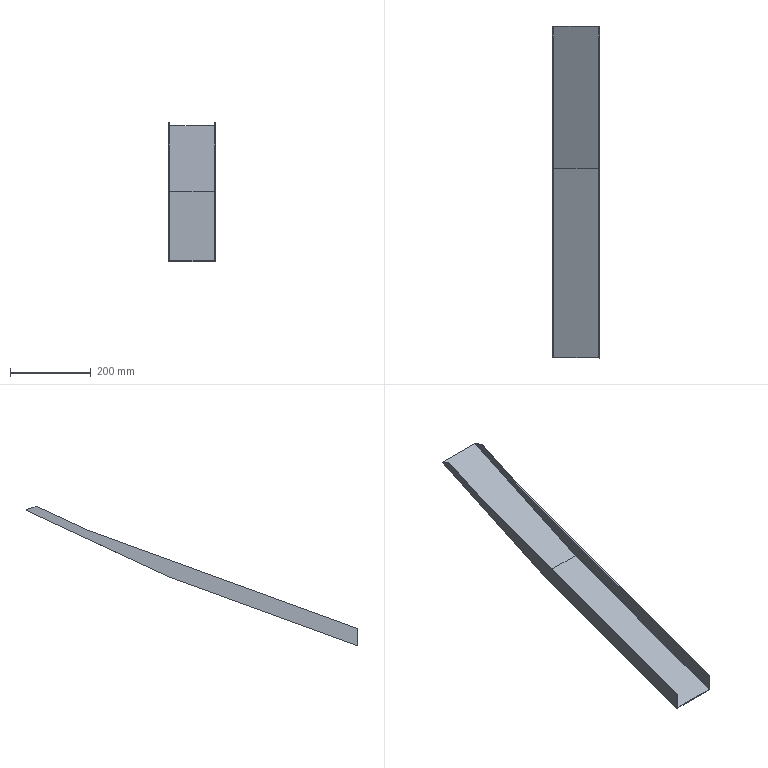Part | NX | features solid 2 | 1 solid | 16 faces | box 115.013 x 820.651 x 345.175 mm | volume 314941 mm3 | plane 16
STEP:
#1=CARTESIAN_POINT('',(53.,-0.1941,-173.187));
#2=VERTEX_POINT('',#1);
#3=CARTESIAN_POINT('',(-60.,-0.1961,-173.178));
#4=VERTEX_POINT('',#3);
#5=CARTESIAN_POINT('',(55.,-0.194,-173.187));
#6=DIRECTION('',(-1.,-0.00001764,0.00007989));
#7=VECTOR('',#6,1000.);
#8=LINE('',#5,#7);
#9=EDGE_CURVE('',#2,#4,#8,.T.);
#10=ORIENTED_EDGE('',*,*,#9,.F.);
#11=CARTESIAN_POINT('',(55.,-0.194,-173.187));
#12=VERTEX_POINT('',#11);
#13=CARTESIAN_POINT('',(55.,-0.194,-173.187));
#14=DIRECTION('',(-1.,-0.00001764,0.00007989));
#15=VECTOR('',#14,1000.);
#16=LINE('',#13,#15);
#17=EDGE_CURVE('',#12,#2,#16,.T.);
#18=ORIENTED_EDGE('',*,*,#17,.F.);
#19=CARTESIAN_POINT('',(55.,0.6512,-175.));
#20=VERTEX_POINT('',#19);
#21=CARTESIAN_POINT('',(54.999,6.339,-187.197));
#22=DIRECTION('',(-0.00008156,0.4226,-0.9063));
#23=VECTOR('',#22,1000.);
#24=LINE('',#21,#23);
#25=EDGE_CURVE('',#12,#20,#24,.T.);
#26=ORIENTED_EDGE('',*,*,#25,.T.);
#27=CARTESIAN_POINT('',(-60.,0.6492,-174.991));
#28=VERTEX_POINT('',#27);
#29=CARTESIAN_POINT('',(55.,0.6512,-175.));
#30=DIRECTION('',(-1.,-0.00001764,0.00007989));
#31=VECTOR('',#30,1000.);
#32=LINE('',#29,#31);
#33=EDGE_CURVE('',#20,#28,#32,.T.);
#34=ORIENTED_EDGE('',*,*,#33,.T.);
#35=CARTESIAN_POINT('',(-60.001,6.337,-187.187));
#36=DIRECTION('',(-0.00008156,0.4226,-0.9063));
#37=VECTOR('',#36,1000.);
#38=LINE('',#35,#37);
#39=EDGE_CURVE('',#4,#28,#38,.T.);
#40=ORIENTED_EDGE('',*,*,#39,.F.);
#41=EDGE_LOOP('',(#10,#18,#26,#34,#40));
#42=FACE_BOUND('',#41,.T.);
#43=CARTESIAN_POINT('',(55.,0.6512,-175.));
#44=DIRECTION('',(-0.00001778,-0.9063,-0.4226));
#45=DIRECTION('',(-1.,-0.00001836,0.00008143));
#46=AXIS2_PLACEMENT_3D('',#43,#44,#45);
#47=PLANE('',#46);
#48=ADVANCED_FACE('',(#42),#47,.F.);
#49=CARTESIAN_POINT('',(-60.007,-350.766,-338.858));
#50=VERTEX_POINT('',#49);
#51=CARTESIAN_POINT('',(-60.004,-190.561,-264.153));
#52=DIRECTION('',(-0.00001778,-0.9063,-0.4226));
#53=VECTOR('',#52,1000.);
#54=LINE('',#51,#53);
#55=EDGE_CURVE('',#28,#50,#54,.T.);
#56=ORIENTED_EDGE('',*,*,#55,.T.);
#57=CARTESIAN_POINT('',(-60.012,-820.,-509.646));
#58=VERTEX_POINT('',#57);
#59=CARTESIAN_POINT('',(-60.005,-184.189,-278.229));
#60=DIRECTION('',(-0.0000106,-0.9397,-0.342));
#61=VECTOR('',#60,1000.);
#62=LINE('',#59,#61);
#63=EDGE_CURVE('',#58,#50,#62,.F.);
#64=ORIENTED_EDGE('',*,*,#63,.F.);
#65=CARTESIAN_POINT('',(-60.009,-820.,-467.078));
#66=VERTEX_POINT('',#65);
#67=CARTESIAN_POINT('',(-60.028,-820.,-699.908));
#68=DIRECTION('',(-0.00008143,0.,-1.));
#69=VECTOR('',#68,1000.);
#70=LINE('',#67,#69);
#71=EDGE_CURVE('',#58,#66,#70,.F.);
#72=ORIENTED_EDGE('',*,*,#71,.T.);
#73=CARTESIAN_POINT('',(-60.001,-150.453,-223.383));
#74=VERTEX_POINT('',#73);
#75=CARTESIAN_POINT('',(-60.002,-197.87,-240.642));
#76=DIRECTION('',(0.0000106,0.9397,0.342));
#77=VECTOR('',#76,1000.);
#78=LINE('',#75,#77);
#79=EDGE_CURVE('',#66,#74,#78,.T.);
#80=ORIENTED_EDGE('',*,*,#79,.T.);
#81=CARTESIAN_POINT('',(-59.999,-24.136,-164.481));
#82=VERTEX_POINT('',#81);
#83=CARTESIAN_POINT('',(-59.998,-7.823,-156.874));
#84=DIRECTION('',(-0.00001778,-0.9063,-0.4226));
#85=VECTOR('',#84,1000.);
#86=LINE('',#83,#85);
#87=EDGE_CURVE('',#82,#74,#86,.T.);
#88=ORIENTED_EDGE('',*,*,#87,.F.);
#89=CARTESIAN_POINT('',(-60.,-0.2158,-173.187));
#90=VERTEX_POINT('',#89);
#91=CARTESIAN_POINT('',(-59.97,-615.968,50.928));
#92=DIRECTION('',(-0.0000451,0.9397,-0.342));
#93=VECTOR('',#92,1000.);
#94=LINE('',#91,#93);
#95=EDGE_CURVE('',#82,#90,#94,.T.);
#96=ORIENTED_EDGE('',*,*,#95,.T.);
#97=CARTESIAN_POINT('',(-60.004,-191.406,-262.341));
#98=DIRECTION('',(-0.00001778,-0.9063,-0.4226));
#99=VECTOR('',#98,1000.);
#100=LINE('',#97,#99);
#101=EDGE_CURVE('',#4,#90,#100,.T.);
#102=ORIENTED_EDGE('',*,*,#101,.F.);
#103=ORIENTED_EDGE('',*,*,#39,.T.);
#104=EDGE_LOOP('',(#56,#64,#72,#80,#88,#96,#102,#103));
#105=FACE_BOUND('',#104,.T.);
#106=CARTESIAN_POINT('',(-60.005,-184.873,-276.35));
#107=DIRECTION('',(1.,0.00001836,-0.00008143));
#108=DIRECTION('',(-0.00008143,0.,-1.));
#109=AXIS2_PLACEMENT_3D('',#106,#107,#108);
#110=PLANE('',#109);
#111=ADVANCED_FACE('',(#105),#110,.F.);
#112=CARTESIAN_POINT('',(-58.007,-350.766,-338.859));
#113=VERTEX_POINT('',#112);
#114=CARTESIAN_POINT('',(-60.007,-350.766,-338.858));
#115=CARTESIAN_POINT('',(-59.34,-350.766,-338.858));
#116=CARTESIAN_POINT('',(-58.674,-350.766,-338.859));
#117=CARTESIAN_POINT('',(-58.007,-350.766,-338.859));
#118=B_SPLINE_CURVE_WITH_KNOTS('',3,(#114,#115,#116,#117),.UNSPECIFIED.,.F.,.F.,(4,4),(0.,1.),.UNSPECIFIED.);
#119=EDGE_CURVE('',#50,#113,#118,.T.);
#120=ORIENTED_EDGE('',*,*,#119,.T.);
#121=CARTESIAN_POINT('',(52.993,-350.766,-338.868));
#122=VERTEX_POINT('',#121);
#123=CARTESIAN_POINT('',(64.99,-350.766,-338.869));
#124=DIRECTION('',(1.,0.,-0.00008812));
#125=VECTOR('',#124,1000.);
#126=LINE('',#123,#125);
#127=EDGE_CURVE('',#113,#122,#126,.T.);
#128=ORIENTED_EDGE('',*,*,#127,.T.);
#129=CARTESIAN_POINT('',(54.993,-350.766,-338.869));
#130=VERTEX_POINT('',#129);
#131=CARTESIAN_POINT('',(52.993,-350.766,-338.868));
#132=CARTESIAN_POINT('',(53.66,-350.766,-338.868));
#133=CARTESIAN_POINT('',(54.326,-350.766,-338.869));
#134=CARTESIAN_POINT('',(54.993,-350.766,-338.869));
#135=B_SPLINE_CURVE_WITH_KNOTS('',3,(#131,#132,#133,#134),.UNSPECIFIED.,.F.,.F.,(4,4),(0.,1.),.UNSPECIFIED.);
#136=EDGE_CURVE('',#122,#130,#135,.T.);
#137=ORIENTED_EDGE('',*,*,#136,.T.);
#138=CARTESIAN_POINT('',(54.988,-820.,-509.656));
#139=VERTEX_POINT('',#138);
#140=CARTESIAN_POINT('',(54.995,-184.187,-278.239));
#141=DIRECTION('',(-0.0000106,-0.9397,-0.342));
#142=VECTOR('',#141,1000.);
#143=LINE('',#140,#142);
#144=EDGE_CURVE('',#139,#130,#143,.F.);
#145=ORIENTED_EDGE('',*,*,#144,.F.);
#146=CARTESIAN_POINT('',(1065.017,-820.,-509.745));
#147=DIRECTION('',(1.,0.,-0.00008812));
#148=VECTOR('',#147,1000.);
#149=LINE('',#146,#148);
#150=EDGE_CURVE('',#139,#58,#149,.F.);
#151=ORIENTED_EDGE('',*,*,#150,.T.);
#152=ORIENTED_EDGE('',*,*,#63,.T.);
#153=EDGE_LOOP('',(#120,#128,#137,#145,#151,#152));
#154=FACE_BOUND('',#153,.T.);
#155=CARTESIAN_POINT('',(64.995,-184.187,-278.24));
#156=DIRECTION('',(0.0000828,-0.342,0.9397));
#157=DIRECTION('',(1.,0.00001836,-0.00008143));
#158=AXIS2_PLACEMENT_3D('',#155,#156,#157);
#159=PLANE('',#158);
#160=ADVANCED_FACE('',(#154),#159,.F.);
#161=CARTESIAN_POINT('',(54.991,-820.,-467.089));
#162=VERTEX_POINT('',#161);
#163=CARTESIAN_POINT('',(54.972,-820.,-699.918));
#164=DIRECTION('',(-0.00008143,0.,-1.));
#165=VECTOR('',#164,1000.);
#166=LINE('',#163,#165);
#167=EDGE_CURVE('',#162,#139,#166,.T.);
#168=ORIENTED_EDGE('',*,*,#167,.T.);
#169=ORIENTED_EDGE('',*,*,#144,.T.);
#170=CARTESIAN_POINT('',(54.996,-190.559,-264.163));
#171=DIRECTION('',(-0.00001778,-0.9063,-0.4226));
#172=VECTOR('',#171,1000.);
#173=LINE('',#170,#172);
#174=EDGE_CURVE('',#20,#130,#173,.T.);
#175=ORIENTED_EDGE('',*,*,#174,.F.);
#176=ORIENTED_EDGE('',*,*,#25,.F.);
#177=CARTESIAN_POINT('',(55.001,-24.115,-164.481));
#178=VERTEX_POINT('',#177);
#179=CARTESIAN_POINT('',(55.,1.135,-173.671));
#180=DIRECTION('',(-0.0000451,0.9397,-0.342));
#181=VECTOR('',#180,1000.);
#182=LINE('',#179,#181);
#183=EDGE_CURVE('',#12,#178,#182,.F.);
#184=ORIENTED_EDGE('',*,*,#183,.T.);
#185=CARTESIAN_POINT('',(54.999,-150.453,-223.393));
#186=VERTEX_POINT('',#185);
#187=CARTESIAN_POINT('',(55.002,-7.801,-156.874));
#188=DIRECTION('',(-0.00001778,-0.9063,-0.4226));
#189=VECTOR('',#188,1000.);
#190=LINE('',#187,#189);
#191=EDGE_CURVE('',#178,#186,#190,.T.);
#192=ORIENTED_EDGE('',*,*,#191,.T.);
#193=CARTESIAN_POINT('',(54.991,-833.681,-472.068));
#194=DIRECTION('',(0.0000106,0.9397,0.342));
#195=VECTOR('',#194,1000.);
#196=LINE('',#193,#195);
#197=EDGE_CURVE('',#162,#186,#196,.T.);
#198=ORIENTED_EDGE('',*,*,#197,.F.);
#199=EDGE_LOOP('',(#168,#169,#175,#176,#184,#192,#198));
#200=FACE_BOUND('',#199,.T.);
#201=CARTESIAN_POINT('',(54.995,-184.871,-276.359));
#202=DIRECTION('',(1.,0.00001836,-0.00008143));
#203=DIRECTION('',(-0.00008143,0.,-1.));
#204=AXIS2_PLACEMENT_3D('',#201,#202,#203);
#205=PLANE('',#204);
#206=ADVANCED_FACE('',(#200),#205,.T.);
#207=CARTESIAN_POINT('',(-58.007,-351.532,-337.009));
#208=VERTEX_POINT('',#207);
#209=CARTESIAN_POINT('',(-58.,-0.2157,-173.188));
#210=VERTEX_POINT('',#209);
#211=CARTESIAN_POINT('',(-58.004,-191.111,-262.203));
#212=DIRECTION('',(-0.00001778,-0.9063,-0.4226));
#213=VECTOR('',#212,1000.);
#214=LINE('',#211,#213);
#215=EDGE_CURVE('',#208,#210,#214,.F.);
#216=ORIENTED_EDGE('',*,*,#215,.F.);
#217=CARTESIAN_POINT('',(52.993,-351.532,-337.019));
#218=VERTEX_POINT('',#217);
#219=CARTESIAN_POINT('',(64.99,-351.532,-337.02));
#220=DIRECTION('',(-1.,0.,0.00008812));
#221=VECTOR('',#220,1000.);
#222=LINE('',#219,#221);
#223=EDGE_CURVE('',#208,#218,#222,.F.);
#224=ORIENTED_EDGE('',*,*,#223,.T.);
#225=CARTESIAN_POINT('',(52.996,-191.109,-262.212));
#226=DIRECTION('',(0.00001778,0.9063,0.4226));
#227=VECTOR('',#226,1000.);
#228=LINE('',#225,#227);
#229=EDGE_CURVE('',#2,#218,#228,.F.);
#230=ORIENTED_EDGE('',*,*,#229,.F.);
#231=ORIENTED_EDGE('',*,*,#9,.T.);
#232=ORIENTED_EDGE('',*,*,#101,.T.);
#233=CARTESIAN_POINT('',(-60.,-0.2158,-173.187));
#234=DIRECTION('',(-1.,-0.00001836,0.00008143));
#235=VECTOR('',#234,1000.);
#236=LINE('',#233,#235);
#237=EDGE_CURVE('',#90,#210,#236,.F.);
#238=ORIENTED_EDGE('',*,*,#237,.T.);
#239=EDGE_LOOP('',(#216,#224,#230,#231,#232,#238));
#240=FACE_BOUND('',#239,.T.);
#241=CARTESIAN_POINT('',(64.996,-191.109,-262.213));
#242=DIRECTION('',(0.00007986,-0.4226,0.9063));
#243=DIRECTION('',(1.,0.0000177,-0.00007986));
#244=AXIS2_PLACEMENT_3D('',#241,#242,#243);
#245=PLANE('',#244);
#246=ADVANCED_FACE('',(#240),#245,.T.);
#247=ORIENTED_EDGE('',*,*,#119,.F.);
#248=ORIENTED_EDGE('',*,*,#55,.F.);
#249=ORIENTED_EDGE('',*,*,#33,.F.);
#250=ORIENTED_EDGE('',*,*,#174,.T.);
#251=ORIENTED_EDGE('',*,*,#136,.F.);
#252=ORIENTED_EDGE('',*,*,#127,.F.);
#253=EDGE_LOOP('',(#247,#248,#249,#250,#251,#252));
#254=FACE_BOUND('',#253,.T.);
#255=CARTESIAN_POINT('',(64.996,-190.263,-264.026));
#256=DIRECTION('',(0.00007986,-0.4226,0.9063));
#257=DIRECTION('',(1.,0.0000177,-0.00007986));
#258=AXIS2_PLACEMENT_3D('',#255,#256,#257);
#259=PLANE('',#258);
#260=ADVANCED_FACE('',(#254),#259,.F.);
#261=ORIENTED_EDGE('',*,*,#71,.F.);
#262=ORIENTED_EDGE('',*,*,#150,.F.);
#263=ORIENTED_EDGE('',*,*,#167,.F.);
#264=CARTESIAN_POINT('',(52.991,-820.,-467.088));
#265=VERTEX_POINT('',#264);
#266=CARTESIAN_POINT('',(54.992,-820.,-467.089));
#267=DIRECTION('',(-1.,0.,0.00008812));
#268=VECTOR('',#267,1000.);
#269=LINE('',#266,#268);
#270=EDGE_CURVE('',#265,#162,#269,.F.);
#271=ORIENTED_EDGE('',*,*,#270,.F.);
#272=CARTESIAN_POINT('',(52.988,-820.,-507.527));
#273=VERTEX_POINT('',#272);
#274=CARTESIAN_POINT('',(52.972,-820.,-699.918));
#275=DIRECTION('',(-0.00008143,0.,-1.));
#276=VECTOR('',#275,1000.);
#277=LINE('',#274,#276);
#278=EDGE_CURVE('',#273,#265,#277,.F.);
#279=ORIENTED_EDGE('',*,*,#278,.F.);
#280=CARTESIAN_POINT('',(-58.012,-820.,-507.517));
#281=VERTEX_POINT('',#280);
#282=CARTESIAN_POINT('',(1065.017,-820.,-507.616));
#283=DIRECTION('',(1.,0.,-0.00008812));
#284=VECTOR('',#283,1000.);
#285=LINE('',#282,#284);
#286=EDGE_CURVE('',#273,#281,#285,.F.);
#287=ORIENTED_EDGE('',*,*,#286,.T.);
#288=CARTESIAN_POINT('',(-58.009,-820.,-467.079));
#289=VERTEX_POINT('',#288);
#290=CARTESIAN_POINT('',(-58.028,-820.,-699.909));
#291=DIRECTION('',(0.00008143,0.,1.));
#292=VECTOR('',#291,1000.);
#293=LINE('',#290,#292);
#294=EDGE_CURVE('',#289,#281,#293,.F.);
#295=ORIENTED_EDGE('',*,*,#294,.F.);
#296=CARTESIAN_POINT('',(1065.021,-820.,-467.178));
#297=DIRECTION('',(-1.,0.,0.00008812));
#298=VECTOR('',#297,1000.);
#299=LINE('',#296,#298);
#300=EDGE_CURVE('',#66,#289,#299,.F.);
#301=ORIENTED_EDGE('',*,*,#300,.F.);
#302=EDGE_LOOP('',(#261,#262,#263,#271,#279,#287,#295,#301));
#303=FACE_BOUND('',#302,.T.);
#304=CARTESIAN_POINT('',(1065.,-820.,-700.));
#305=DIRECTION('',(0.,1.,0.));
#306=DIRECTION('',(-1.,0.,0.));
#307=AXIS2_PLACEMENT_3D('',#304,#305,#306);
#308=PLANE('',#307);
#309=ADVANCED_FACE('',(#303),#308,.F.);
#310=CARTESIAN_POINT('',(-58.005,-184.873,-276.35));
#311=DIRECTION('',(-0.0000106,-0.9397,-0.342));
#312=VECTOR('',#311,1000.);
#313=LINE('',#310,#312);
#314=EDGE_CURVE('',#281,#208,#313,.F.);
#315=ORIENTED_EDGE('',*,*,#314,.F.);
#316=ORIENTED_EDGE('',*,*,#286,.F.);
#317=CARTESIAN_POINT('',(52.995,-184.871,-276.359));
#318=DIRECTION('',(0.0000106,0.9397,0.342));
#319=VECTOR('',#318,1000.);
#320=LINE('',#317,#319);
#321=EDGE_CURVE('',#218,#273,#320,.F.);
#322=ORIENTED_EDGE('',*,*,#321,.F.);
#323=ORIENTED_EDGE('',*,*,#223,.F.);
#324=EDGE_LOOP('',(#315,#316,#322,#323));
#325=FACE_BOUND('',#324,.T.);
#326=CARTESIAN_POINT('',(64.995,-184.871,-276.36));
#327=DIRECTION('',(0.0000828,-0.342,0.9397));
#328=DIRECTION('',(1.,0.00001836,-0.00008143));
#329=AXIS2_PLACEMENT_3D('',#326,#327,#328);
#330=PLANE('',#329);
#331=ADVANCED_FACE('',(#325),#330,.T.);
#332=CARTESIAN_POINT('',(53.001,-24.115,-164.481));
#333=VERTEX_POINT('',#332);
#334=CARTESIAN_POINT('',(53.03,-615.962,50.934));
#335=DIRECTION('',(-0.0000451,0.9397,-0.342));
#336=VECTOR('',#335,1000.);
#337=LINE('',#334,#336);
#338=EDGE_CURVE('',#333,#2,#337,.T.);
#339=ORIENTED_EDGE('',*,*,#338,.T.);
#340=ORIENTED_EDGE('',*,*,#229,.T.);
#341=ORIENTED_EDGE('',*,*,#321,.T.);
#342=ORIENTED_EDGE('',*,*,#278,.T.);
#343=CARTESIAN_POINT('',(52.999,-150.453,-223.393));
#344=VERTEX_POINT('',#343);
#345=CARTESIAN_POINT('',(52.991,-833.681,-472.068));
#346=DIRECTION('',(-0.0000106,-0.9397,-0.342));
#347=VECTOR('',#346,1000.);
#348=LINE('',#345,#347);
#349=EDGE_CURVE('',#265,#344,#348,.F.);
#350=ORIENTED_EDGE('',*,*,#349,.T.);
#351=CARTESIAN_POINT('',(53.002,-7.801,-156.874));
#352=DIRECTION('',(-0.00001778,-0.9063,-0.4226));
#353=VECTOR('',#352,1000.);
#354=LINE('',#351,#353);
#355=EDGE_CURVE('',#333,#344,#354,.T.);
#356=ORIENTED_EDGE('',*,*,#355,.F.);
#357=EDGE_LOOP('',(#339,#340,#341,#342,#350,#356));
#358=FACE_BOUND('',#357,.T.);
#359=CARTESIAN_POINT('',(52.988,-820.,-509.656));
#360=DIRECTION('',(1.,0.00001836,-0.00008143));
#361=DIRECTION('',(0.0000106,0.9397,0.342));
#362=AXIS2_PLACEMENT_3D('',#359,#360,#361);
#363=PLANE('',#362);
#364=ADVANCED_FACE('',(#358),#363,.F.);
#365=ORIENTED_EDGE('',*,*,#191,.F.);
#366=CARTESIAN_POINT('',(53.001,-24.115,-164.481));
#367=DIRECTION('',(-1.,-0.00001836,0.00008143));
#368=VECTOR('',#367,1000.);
#369=LINE('',#366,#368);
#370=EDGE_CURVE('',#178,#333,#369,.T.);
#371=ORIENTED_EDGE('',*,*,#370,.T.);
#372=ORIENTED_EDGE('',*,*,#355,.T.);
#373=CARTESIAN_POINT('',(54.999,-150.453,-223.393));
#374=DIRECTION('',(-1.,-0.00001836,0.00008143));
#375=VECTOR('',#374,1000.);
#376=LINE('',#373,#375);
#377=EDGE_CURVE('',#186,#344,#376,.T.);
#378=ORIENTED_EDGE('',*,*,#377,.F.);
#379=EDGE_LOOP('',(#365,#371,#372,#378));
#380=FACE_BOUND('',#379,.T.);
#381=CARTESIAN_POINT('',(55.002,-7.801,-156.874));
#382=DIRECTION('',(-0.00008156,0.4226,-0.9063));
#383=DIRECTION('',(0.,0.9063,0.4226));
#384=AXIS2_PLACEMENT_3D('',#381,#382,#383);
#385=PLANE('',#384);
#386=ADVANCED_FACE('',(#380),#385,.F.);
#387=ORIENTED_EDGE('',*,*,#349,.F.);
#388=ORIENTED_EDGE('',*,*,#270,.T.);
#389=ORIENTED_EDGE('',*,*,#197,.T.);
#390=ORIENTED_EDGE('',*,*,#377,.T.);
#391=EDGE_LOOP('',(#387,#388,#389,#390));
#392=FACE_BOUND('',#391,.T.);
#393=CARTESIAN_POINT('',(54.991,-833.681,-472.068));
#394=DIRECTION('',(0.0000828,-0.342,0.9397));
#395=DIRECTION('',(0.,-0.9397,-0.342));
#396=AXIS2_PLACEMENT_3D('',#393,#394,#395);
#397=PLANE('',#396);
#398=ADVANCED_FACE('',(#392),#397,.T.);
#399=ORIENTED_EDGE('',*,*,#183,.F.);
#400=ORIENTED_EDGE('',*,*,#17,.T.);
#401=ORIENTED_EDGE('',*,*,#338,.F.);
#402=ORIENTED_EDGE('',*,*,#370,.F.);
#403=EDGE_LOOP('',(#399,#400,#401,#402));
#404=FACE_BOUND('',#403,.T.);
#405=CARTESIAN_POINT('',(55.001,-24.115,-164.481));
#406=DIRECTION('',(-0.00007025,-0.342,-0.9397));
#407=DIRECTION('',(0.,0.9397,-0.342));
#408=AXIS2_PLACEMENT_3D('',#405,#406,#407);
#409=PLANE('',#408);
#410=ADVANCED_FACE('',(#404),#409,.F.);
#411=CARTESIAN_POINT('',(-57.999,-24.136,-164.481));
#412=VERTEX_POINT('',#411);
#413=CARTESIAN_POINT('',(-58.001,-150.453,-223.383));
#414=VERTEX_POINT('',#413);
#415=CARTESIAN_POINT('',(-57.998,-7.823,-156.874));
#416=DIRECTION('',(-0.00001778,-0.9063,-0.4226));
#417=VECTOR('',#416,1000.);
#418=LINE('',#415,#417);
#419=EDGE_CURVE('',#412,#414,#418,.T.);
#420=ORIENTED_EDGE('',*,*,#419,.F.);
#421=CARTESIAN_POINT('',(-59.999,-24.136,-164.481));
#422=DIRECTION('',(-1.,-0.00001836,0.00008143));
#423=VECTOR('',#422,1000.);
#424=LINE('',#421,#423);
#425=EDGE_CURVE('',#412,#82,#424,.T.);
#426=ORIENTED_EDGE('',*,*,#425,.T.);
#427=ORIENTED_EDGE('',*,*,#87,.T.);
#428=CARTESIAN_POINT('',(-60.001,-150.453,-223.383));
#429=DIRECTION('',(1.,0.00001836,-0.00008143));
#430=VECTOR('',#429,1000.);
#431=LINE('',#428,#430);
#432=EDGE_CURVE('',#74,#414,#431,.T.);
#433=ORIENTED_EDGE('',*,*,#432,.T.);
#434=EDGE_LOOP('',(#420,#426,#427,#433));
#435=FACE_BOUND('',#434,.T.);
#436=CARTESIAN_POINT('',(-59.998,-7.823,-156.874));
#437=DIRECTION('',(0.00008156,-0.4226,0.9063));
#438=DIRECTION('',(0.,-0.9063,-0.4226));
#439=AXIS2_PLACEMENT_3D('',#436,#437,#438);
#440=PLANE('',#439);
#441=ADVANCED_FACE('',(#435),#440,.T.);
#442=ORIENTED_EDGE('',*,*,#79,.F.);
#443=ORIENTED_EDGE('',*,*,#300,.T.);
#444=CARTESIAN_POINT('',(-57.999,-1.494,-169.167));
#445=DIRECTION('',(-0.0000106,-0.9397,-0.342));
#446=VECTOR('',#445,1000.);
#447=LINE('',#444,#446);
#448=EDGE_CURVE('',#289,#414,#447,.F.);
#449=ORIENTED_EDGE('',*,*,#448,.T.);
#450=ORIENTED_EDGE('',*,*,#432,.F.);
#451=EDGE_LOOP('',(#442,#443,#449,#450));
#452=FACE_BOUND('',#451,.T.);
#453=CARTESIAN_POINT('',(-60.009,-833.681,-472.058));
#454=DIRECTION('',(-0.0000828,0.342,-0.9397));
#455=DIRECTION('',(0.,0.9397,0.342));
#456=AXIS2_PLACEMENT_3D('',#453,#454,#455);
#457=PLANE('',#456);
#458=ADVANCED_FACE('',(#452),#457,.F.);
#459=ORIENTED_EDGE('',*,*,#314,.T.);
#460=ORIENTED_EDGE('',*,*,#215,.T.);
#461=CARTESIAN_POINT('',(-58.,1.113,-173.671));
#462=DIRECTION('',(-0.0000451,0.9397,-0.342));
#463=VECTOR('',#462,1000.);
#464=LINE('',#461,#463);
#465=EDGE_CURVE('',#210,#412,#464,.F.);
#466=ORIENTED_EDGE('',*,*,#465,.T.);
#467=ORIENTED_EDGE('',*,*,#419,.T.);
#468=ORIENTED_EDGE('',*,*,#448,.F.);
#469=ORIENTED_EDGE('',*,*,#294,.T.);
#470=EDGE_LOOP('',(#459,#460,#466,#467,#468,#469));
#471=FACE_BOUND('',#470,.T.);
#472=CARTESIAN_POINT('',(-58.,0.6295,-175.));
#473=DIRECTION('',(-1.,-0.00001836,0.00008143));
#474=DIRECTION('',(-0.00001778,-0.9063,-0.4226));
#475=AXIS2_PLACEMENT_3D('',#472,#473,#474);
#476=PLANE('',#475);
#477=ADVANCED_FACE('',(#471),#476,.F.);
#478=ORIENTED_EDGE('',*,*,#95,.F.);
#479=ORIENTED_EDGE('',*,*,#425,.F.);
#480=ORIENTED_EDGE('',*,*,#465,.F.);
#481=ORIENTED_EDGE('',*,*,#237,.F.);
#482=EDGE_LOOP('',(#478,#479,#480,#481));
#483=FACE_BOUND('',#482,.T.);
#484=CARTESIAN_POINT('',(-60.,-0.2158,-173.187));
#485=DIRECTION('',(0.00007025,0.342,0.9397));
#486=DIRECTION('',(0.,-0.9397,0.342));
#487=AXIS2_PLACEMENT_3D('',#484,#485,#486);
#488=PLANE('',#487);
#489=ADVANCED_FACE('',(#483),#488,.T.);
#490=CLOSED_SHELL('',(#48,#111,#160,#206,#246,#260,#309,#331,#364,#386,#398,#410,#441,#458,#477,#489));
#491=MANIFOLD_SOLID_BREP('',#490);
#492=(LENGTH_UNIT()NAMED_UNIT(*)SI_UNIT(.MILLI.,.METRE.));
#493=UNCERTAINTY_MEASURE_WITH_UNIT(LENGTH_MEASURE(0.0508),#492,'','');
#494=(NAMED_UNIT(*)PLANE_ANGLE_UNIT()SI_UNIT($,.RADIAN.));
#495=(NAMED_UNIT(*)SI_UNIT($,.STERADIAN.)SOLID_ANGLE_UNIT());
#496=(GEOMETRIC_REPRESENTATION_CONTEXT(3)GLOBAL_UNCERTAINTY_ASSIGNED_CONTEXT((#493))GLOBAL_UNIT_ASSIGNED_CONTEXT((#492,#494,#495))REPRESENTATION_CONTEXT('',''));
#497=ADVANCED_BREP_SHAPE_REPRESENTATION('',(#491),#496);